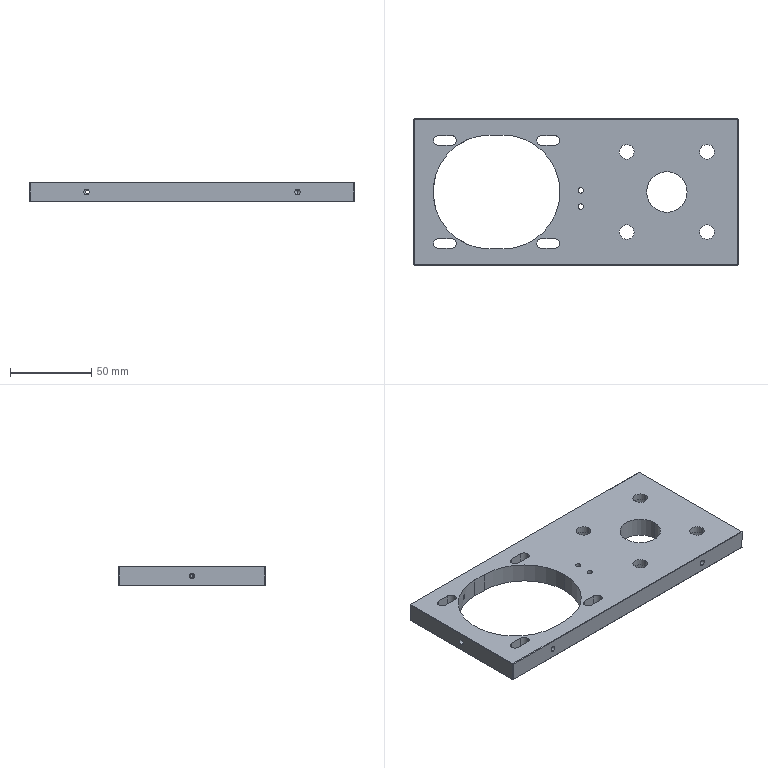Part | SolidWorks | features BaseBody 1 | 1 solid | 95 faces | box 200 x 90 x 12 mm | volume 145701 mm3 | cylinder 49 | plane 32 | cone 14 | commonest cylinder face diameters 6 x12 3.3 x8 3.4 x8 9 x8 15 x8 70.2 x3